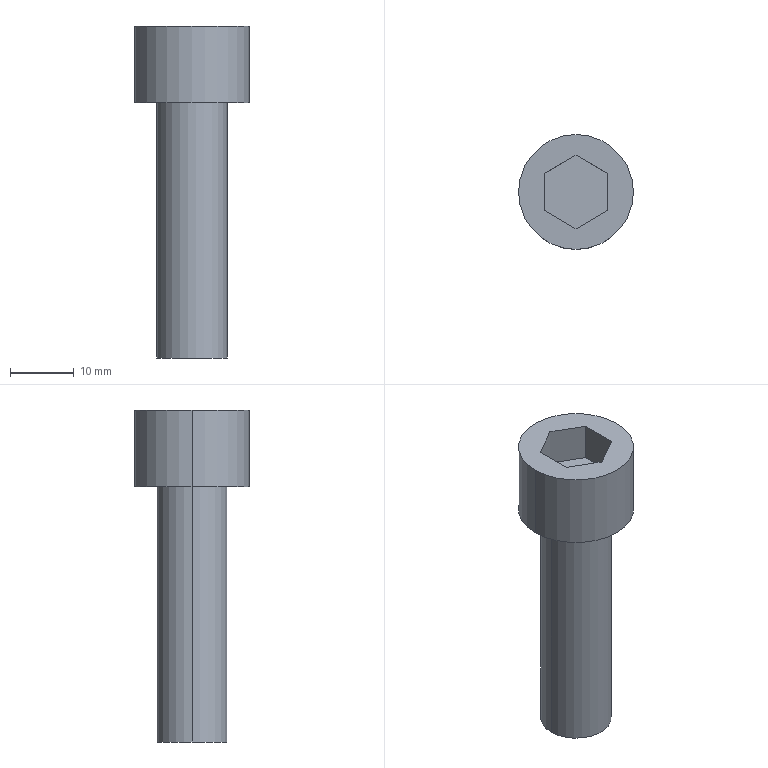Part | SolidWorks | features ICE 2, Extrusion 1 | 1 solid | 14 faces | box 18 x 18 x 52 mm | volume 6335 mm3 | plane 10 | cylinder 4 | commonest cylinder face diameters 11 x2 18 x2
STEP:
#1=CARTESIAN_POINT('',(9.,0.,52.));
#2=VERTEX_POINT('',#1);
#3=CARTESIAN_POINT('',(-9.,0.,52.));
#4=VERTEX_POINT('',#3);
#5=CARTESIAN_POINT('',(0.,0.,52.));
#6=DIRECTION('',(0.,0.,1.));
#7=DIRECTION('',(1.,0.,0.));
#8=AXIS2_PLACEMENT_3D('',#5,#6,#7);
#9=CIRCLE('',#8,9.);
#10=EDGE_CURVE('',#2,#4,#9,.T.);
#11=ORIENTED_EDGE('',*,*,#10,.F.);
#12=CARTESIAN_POINT('',(9.,0.,40.));
#13=VERTEX_POINT('',#12);
#14=CARTESIAN_POINT('',(9.,0.,52.));
#15=DIRECTION('',(0.,0.,-1.));
#16=VECTOR('',#15,1000.);
#17=LINE('',#14,#16);
#18=EDGE_CURVE('',#2,#13,#17,.T.);
#19=ORIENTED_EDGE('',*,*,#18,.T.);
#20=CARTESIAN_POINT('',(-9.,0.,40.));
#21=VERTEX_POINT('',#20);
#22=CARTESIAN_POINT('',(0.,0.,40.));
#23=DIRECTION('',(0.,0.,1.));
#24=DIRECTION('',(1.,0.,0.));
#25=AXIS2_PLACEMENT_3D('',#22,#23,#24);
#26=CIRCLE('',#25,9.);
#27=EDGE_CURVE('',#13,#21,#26,.T.);
#28=ORIENTED_EDGE('',*,*,#27,.T.);
#29=CARTESIAN_POINT('',(-9.,0.,52.));
#30=DIRECTION('',(0.,0.,-1.));
#31=VECTOR('',#30,1000.);
#32=LINE('',#29,#31);
#33=EDGE_CURVE('',#4,#21,#32,.T.);
#34=ORIENTED_EDGE('',*,*,#33,.F.);
#35=EDGE_LOOP('',(#11,#19,#28,#34));
#36=FACE_OUTER_BOUND('',#35,.T.);
#37=CARTESIAN_POINT('',(0.,0.,52.));
#38=DIRECTION('',(0.,0.,-1.));
#39=DIRECTION('',(-1.,0.,0.));
#40=AXIS2_PLACEMENT_3D('',#37,#38,#39);
#41=CYLINDRICAL_SURFACE('',#40,9.);
#42=ADVANCED_FACE('',(#36),#41,.T.);
#43=CARTESIAN_POINT('',(5.5,0.,40.));
#44=VERTEX_POINT('',#43);
#45=CARTESIAN_POINT('',(-5.5,0.,40.));
#46=VERTEX_POINT('',#45);
#47=CARTESIAN_POINT('',(0.,0.,40.));
#48=DIRECTION('',(0.,0.,1.));
#49=DIRECTION('',(1.,0.,0.));
#50=AXIS2_PLACEMENT_3D('',#47,#48,#49);
#51=CIRCLE('',#50,5.5);
#52=EDGE_CURVE('',#44,#46,#51,.T.);
#53=ORIENTED_EDGE('',*,*,#52,.F.);
#54=CARTESIAN_POINT('',(5.5,0.,0.));
#55=VERTEX_POINT('',#54);
#56=CARTESIAN_POINT('',(5.5,0.,40.));
#57=DIRECTION('',(0.,0.,-1.));
#58=VECTOR('',#57,1000.);
#59=LINE('',#56,#58);
#60=EDGE_CURVE('',#44,#55,#59,.T.);
#61=ORIENTED_EDGE('',*,*,#60,.T.);
#62=CARTESIAN_POINT('',(-5.5,0.,0.));
#63=VERTEX_POINT('',#62);
#64=CARTESIAN_POINT('',(0.,0.,0.));
#65=DIRECTION('',(0.,0.,1.));
#66=DIRECTION('',(1.,0.,0.));
#67=AXIS2_PLACEMENT_3D('',#64,#65,#66);
#68=CIRCLE('',#67,5.5);
#69=EDGE_CURVE('',#55,#63,#68,.T.);
#70=ORIENTED_EDGE('',*,*,#69,.T.);
#71=CARTESIAN_POINT('',(-5.5,0.,40.));
#72=DIRECTION('',(0.,0.,-1.));
#73=VECTOR('',#72,1000.);
#74=LINE('',#71,#73);
#75=EDGE_CURVE('',#46,#63,#74,.T.);
#76=ORIENTED_EDGE('',*,*,#75,.F.);
#77=EDGE_LOOP('',(#53,#61,#70,#76));
#78=FACE_OUTER_BOUND('',#77,.T.);
#79=CARTESIAN_POINT('',(0.,0.,40.));
#80=DIRECTION('',(0.,0.,-1.));
#81=DIRECTION('',(-1.,0.,0.));
#82=AXIS2_PLACEMENT_3D('',#79,#80,#81);
#83=CYLINDRICAL_SURFACE('',#82,5.5);
#84=ADVANCED_FACE('',(#78),#83,.T.);
#85=ORIENTED_EDGE('',*,*,#60,.F.);
#86=CARTESIAN_POINT('',(0.,0.,40.));
#87=DIRECTION('',(0.,0.,1.));
#88=DIRECTION('',(1.,0.,0.));
#89=AXIS2_PLACEMENT_3D('',#86,#87,#88);
#90=CIRCLE('',#89,5.5);
#91=EDGE_CURVE('',#46,#44,#90,.T.);
#92=ORIENTED_EDGE('',*,*,#91,.F.);
#93=ORIENTED_EDGE('',*,*,#75,.T.);
#94=CARTESIAN_POINT('',(0.,0.,0.));
#95=DIRECTION('',(0.,0.,1.));
#96=DIRECTION('',(1.,0.,0.));
#97=AXIS2_PLACEMENT_3D('',#94,#95,#96);
#98=CIRCLE('',#97,5.5);
#99=EDGE_CURVE('',#63,#55,#98,.T.);
#100=ORIENTED_EDGE('',*,*,#99,.T.);
#101=EDGE_LOOP('',(#85,#92,#93,#100));
#102=FACE_OUTER_BOUND('',#101,.T.);
#103=CARTESIAN_POINT('',(0.,0.,40.));
#104=DIRECTION('',(0.,0.,-1.));
#105=DIRECTION('',(-1.,0.,0.));
#106=AXIS2_PLACEMENT_3D('',#103,#104,#105);
#107=CYLINDRICAL_SURFACE('',#106,5.5);
#108=ADVANCED_FACE('',(#102),#107,.T.);
#109=ORIENTED_EDGE('',*,*,#99,.F.);
#110=ORIENTED_EDGE('',*,*,#69,.F.);
#111=EDGE_LOOP('',(#109,#110));
#112=FACE_OUTER_BOUND('',#111,.T.);
#113=CARTESIAN_POINT('',(0.,0.,0.));
#114=DIRECTION('',(0.,0.,1.));
#115=DIRECTION('',(1.,0.,0.));
#116=AXIS2_PLACEMENT_3D('',#113,#114,#115);
#117=PLANE('',#116);
#118=ADVANCED_FACE('',(#112),#117,.F.);
#119=CARTESIAN_POINT('',(0.,0.,40.));
#120=DIRECTION('',(0.,0.,1.));
#121=DIRECTION('',(1.,0.,0.));
#122=AXIS2_PLACEMENT_3D('',#119,#120,#121);
#123=CIRCLE('',#122,9.);
#124=EDGE_CURVE('',#21,#13,#123,.T.);
#125=ORIENTED_EDGE('',*,*,#124,.F.);
#126=ORIENTED_EDGE('',*,*,#27,.F.);
#127=EDGE_LOOP('',(#125,#126));
#128=FACE_OUTER_BOUND('',#127,.T.);
#129=ORIENTED_EDGE('',*,*,#91,.T.);
#130=ORIENTED_EDGE('',*,*,#52,.T.);
#131=EDGE_LOOP('',(#129,#130));
#132=FACE_BOUND('',#131,.T.);
#133=CARTESIAN_POINT('',(0.,0.,40.));
#134=DIRECTION('',(0.,0.,1.));
#135=DIRECTION('',(1.,0.,0.));
#136=AXIS2_PLACEMENT_3D('',#133,#134,#135);
#137=PLANE('',#136);
#138=ADVANCED_FACE('',(#128,#132),#137,.F.);
#139=ORIENTED_EDGE('',*,*,#18,.F.);
#140=CARTESIAN_POINT('',(0.,0.,52.));
#141=DIRECTION('',(0.,0.,1.));
#142=DIRECTION('',(1.,0.,0.));
#143=AXIS2_PLACEMENT_3D('',#140,#141,#142);
#144=CIRCLE('',#143,9.);
#145=EDGE_CURVE('',#4,#2,#144,.T.);
#146=ORIENTED_EDGE('',*,*,#145,.F.);
#147=ORIENTED_EDGE('',*,*,#33,.T.);
#148=ORIENTED_EDGE('',*,*,#124,.T.);
#149=EDGE_LOOP('',(#139,#146,#147,#148));
#150=FACE_OUTER_BOUND('',#149,.T.);
#151=CARTESIAN_POINT('',(0.,0.,52.));
#152=DIRECTION('',(0.,0.,-1.));
#153=DIRECTION('',(-1.,0.,0.));
#154=AXIS2_PLACEMENT_3D('',#151,#152,#153);
#155=CYLINDRICAL_SURFACE('',#154,9.);
#156=ADVANCED_FACE('',(#150),#155,.T.);
#157=CARTESIAN_POINT('',(5.,2.887,52.));
#158=VERTEX_POINT('',#157);
#159=CARTESIAN_POINT('',(0.,5.774,52.));
#160=VERTEX_POINT('',#159);
#161=CARTESIAN_POINT('',(5.,2.887,52.));
#162=DIRECTION('',(-0.866,0.5,0.));
#163=VECTOR('',#162,1000.);
#164=LINE('',#161,#163);
#165=EDGE_CURVE('',#158,#160,#164,.T.);
#166=ORIENTED_EDGE('',*,*,#165,.F.);
#167=CARTESIAN_POINT('',(5.,-2.887,52.));
#168=VERTEX_POINT('',#167);
#169=CARTESIAN_POINT('',(5.,-2.887,52.));
#170=DIRECTION('',(0.,1.,0.));
#171=VECTOR('',#170,1000.);
#172=LINE('',#169,#171);
#173=EDGE_CURVE('',#168,#158,#172,.T.);
#174=ORIENTED_EDGE('',*,*,#173,.F.);
#175=CARTESIAN_POINT('',(0.,-5.774,52.));
#176=VERTEX_POINT('',#175);
#177=CARTESIAN_POINT('',(0.,-5.774,52.));
#178=DIRECTION('',(0.866,0.5,0.));
#179=VECTOR('',#178,1000.);
#180=LINE('',#177,#179);
#181=EDGE_CURVE('',#176,#168,#180,.T.);
#182=ORIENTED_EDGE('',*,*,#181,.F.);
#183=CARTESIAN_POINT('',(-5.,-2.887,52.));
#184=VERTEX_POINT('',#183);
#185=CARTESIAN_POINT('',(-5.,-2.887,52.));
#186=DIRECTION('',(0.866,-0.5,0.));
#187=VECTOR('',#186,1000.);
#188=LINE('',#185,#187);
#189=EDGE_CURVE('',#184,#176,#188,.T.);
#190=ORIENTED_EDGE('',*,*,#189,.F.);
#191=CARTESIAN_POINT('',(-5.,2.887,52.));
#192=VERTEX_POINT('',#191);
#193=CARTESIAN_POINT('',(-5.,2.887,52.));
#194=DIRECTION('',(0.,-1.,0.));
#195=VECTOR('',#194,1000.);
#196=LINE('',#193,#195);
#197=EDGE_CURVE('',#192,#184,#196,.T.);
#198=ORIENTED_EDGE('',*,*,#197,.F.);
#199=CARTESIAN_POINT('',(0.,5.774,52.));
#200=DIRECTION('',(-0.866,-0.5,0.));
#201=VECTOR('',#200,1000.);
#202=LINE('',#199,#201);
#203=EDGE_CURVE('',#160,#192,#202,.T.);
#204=ORIENTED_EDGE('',*,*,#203,.F.);
#205=EDGE_LOOP('',(#166,#174,#182,#190,#198,#204));
#206=FACE_BOUND('',#205,.T.);
#207=ORIENTED_EDGE('',*,*,#145,.T.);
#208=ORIENTED_EDGE('',*,*,#10,.T.);
#209=EDGE_LOOP('',(#207,#208));
#210=FACE_OUTER_BOUND('',#209,.T.);
#211=CARTESIAN_POINT('',(0.,0.,52.));
#212=DIRECTION('',(0.,0.,1.));
#213=DIRECTION('',(1.,0.,0.));
#214=AXIS2_PLACEMENT_3D('',#211,#212,#213);
#215=PLANE('',#214);
#216=ADVANCED_FACE('',(#206,#210),#215,.T.);
#217=ORIENTED_EDGE('',*,*,#165,.T.);
#218=CARTESIAN_POINT('',(0.,5.774,46.));
#219=VERTEX_POINT('',#218);
#220=CARTESIAN_POINT('',(0.,5.774,46.));
#221=DIRECTION('',(0.,0.,1.));
#222=VECTOR('',#221,1000.);
#223=LINE('',#220,#222);
#224=EDGE_CURVE('',#219,#160,#223,.T.);
#225=ORIENTED_EDGE('',*,*,#224,.F.);
#226=CARTESIAN_POINT('',(5.,2.887,46.));
#227=VERTEX_POINT('',#226);
#228=CARTESIAN_POINT('',(5.,2.887,46.));
#229=DIRECTION('',(-0.866,0.5,0.));
#230=VECTOR('',#229,1000.);
#231=LINE('',#228,#230);
#232=EDGE_CURVE('',#227,#219,#231,.T.);
#233=ORIENTED_EDGE('',*,*,#232,.F.);
#234=CARTESIAN_POINT('',(5.,2.887,46.));
#235=DIRECTION('',(0.,0.,1.));
#236=VECTOR('',#235,1000.);
#237=LINE('',#234,#236);
#238=EDGE_CURVE('',#227,#158,#237,.T.);
#239=ORIENTED_EDGE('',*,*,#238,.T.);
#240=EDGE_LOOP('',(#217,#225,#233,#239));
#241=FACE_OUTER_BOUND('',#240,.T.);
#242=CARTESIAN_POINT('',(5.,2.887,46.));
#243=DIRECTION('',(0.5,0.866,0.));
#244=DIRECTION('',(-0.866,0.5,0.));
#245=AXIS2_PLACEMENT_3D('',#242,#243,#244);
#246=PLANE('',#245);
#247=ADVANCED_FACE('',(#241),#246,.F.);
#248=ORIENTED_EDGE('',*,*,#173,.T.);
#249=ORIENTED_EDGE('',*,*,#238,.F.);
#250=CARTESIAN_POINT('',(5.,-2.887,46.));
#251=VERTEX_POINT('',#250);
#252=CARTESIAN_POINT('',(5.,-2.887,46.));
#253=DIRECTION('',(0.,1.,0.));
#254=VECTOR('',#253,1000.);
#255=LINE('',#252,#254);
#256=EDGE_CURVE('',#251,#227,#255,.T.);
#257=ORIENTED_EDGE('',*,*,#256,.F.);
#258=CARTESIAN_POINT('',(5.,-2.887,46.));
#259=DIRECTION('',(0.,0.,1.));
#260=VECTOR('',#259,1000.);
#261=LINE('',#258,#260);
#262=EDGE_CURVE('',#251,#168,#261,.T.);
#263=ORIENTED_EDGE('',*,*,#262,.T.);
#264=EDGE_LOOP('',(#248,#249,#257,#263));
#265=FACE_OUTER_BOUND('',#264,.T.);
#266=CARTESIAN_POINT('',(5.,-2.887,46.));
#267=DIRECTION('',(1.,0.,0.));
#268=DIRECTION('',(0.,1.,0.));
#269=AXIS2_PLACEMENT_3D('',#266,#267,#268);
#270=PLANE('',#269);
#271=ADVANCED_FACE('',(#265),#270,.F.);
#272=ORIENTED_EDGE('',*,*,#181,.T.);
#273=ORIENTED_EDGE('',*,*,#262,.F.);
#274=CARTESIAN_POINT('',(0.,-5.774,46.));
#275=VERTEX_POINT('',#274);
#276=CARTESIAN_POINT('',(0.,-5.774,46.));
#277=DIRECTION('',(0.866,0.5,0.));
#278=VECTOR('',#277,1000.);
#279=LINE('',#276,#278);
#280=EDGE_CURVE('',#275,#251,#279,.T.);
#281=ORIENTED_EDGE('',*,*,#280,.F.);
#282=CARTESIAN_POINT('',(0.,-5.774,46.));
#283=DIRECTION('',(0.,0.,1.));
#284=VECTOR('',#283,1000.);
#285=LINE('',#282,#284);
#286=EDGE_CURVE('',#275,#176,#285,.T.);
#287=ORIENTED_EDGE('',*,*,#286,.T.);
#288=EDGE_LOOP('',(#272,#273,#281,#287));
#289=FACE_OUTER_BOUND('',#288,.T.);
#290=CARTESIAN_POINT('',(0.,-5.774,46.));
#291=DIRECTION('',(0.5,-0.866,0.));
#292=DIRECTION('',(0.866,0.5,0.));
#293=AXIS2_PLACEMENT_3D('',#290,#291,#292);
#294=PLANE('',#293);
#295=ADVANCED_FACE('',(#289),#294,.F.);
#296=ORIENTED_EDGE('',*,*,#189,.T.);
#297=ORIENTED_EDGE('',*,*,#286,.F.);
#298=CARTESIAN_POINT('',(-5.,-2.887,46.));
#299=VERTEX_POINT('',#298);
#300=CARTESIAN_POINT('',(-5.,-2.887,46.));
#301=DIRECTION('',(0.866,-0.5,0.));
#302=VECTOR('',#301,1000.);
#303=LINE('',#300,#302);
#304=EDGE_CURVE('',#299,#275,#303,.T.);
#305=ORIENTED_EDGE('',*,*,#304,.F.);
#306=CARTESIAN_POINT('',(-5.,-2.887,46.));
#307=DIRECTION('',(0.,0.,1.));
#308=VECTOR('',#307,1000.);
#309=LINE('',#306,#308);
#310=EDGE_CURVE('',#299,#184,#309,.T.);
#311=ORIENTED_EDGE('',*,*,#310,.T.);
#312=EDGE_LOOP('',(#296,#297,#305,#311));
#313=FACE_OUTER_BOUND('',#312,.T.);
#314=CARTESIAN_POINT('',(-5.,-2.887,46.));
#315=DIRECTION('',(-0.5,-0.866,0.));
#316=DIRECTION('',(0.866,-0.5,0.));
#317=AXIS2_PLACEMENT_3D('',#314,#315,#316);
#318=PLANE('',#317);
#319=ADVANCED_FACE('',(#313),#318,.F.);
#320=ORIENTED_EDGE('',*,*,#197,.T.);
#321=ORIENTED_EDGE('',*,*,#310,.F.);
#322=CARTESIAN_POINT('',(-5.,2.887,46.));
#323=VERTEX_POINT('',#322);
#324=CARTESIAN_POINT('',(-5.,2.887,46.));
#325=DIRECTION('',(0.,-1.,0.));
#326=VECTOR('',#325,1000.);
#327=LINE('',#324,#326);
#328=EDGE_CURVE('',#323,#299,#327,.T.);
#329=ORIENTED_EDGE('',*,*,#328,.F.);
#330=CARTESIAN_POINT('',(-5.,2.887,46.));
#331=DIRECTION('',(0.,0.,1.));
#332=VECTOR('',#331,1000.);
#333=LINE('',#330,#332);
#334=EDGE_CURVE('',#323,#192,#333,.T.);
#335=ORIENTED_EDGE('',*,*,#334,.T.);
#336=EDGE_LOOP('',(#320,#321,#329,#335));
#337=FACE_OUTER_BOUND('',#336,.T.);
#338=CARTESIAN_POINT('',(-5.,2.887,46.));
#339=DIRECTION('',(-1.,0.,0.));
#340=DIRECTION('',(0.,0.,1.));
#341=AXIS2_PLACEMENT_3D('',#338,#339,#340);
#342=PLANE('',#341);
#343=ADVANCED_FACE('',(#337),#342,.F.);
#344=ORIENTED_EDGE('',*,*,#203,.T.);
#345=ORIENTED_EDGE('',*,*,#334,.F.);
#346=CARTESIAN_POINT('',(0.,5.774,46.));
#347=DIRECTION('',(-0.866,-0.5,0.));
#348=VECTOR('',#347,1000.);
#349=LINE('',#346,#348);
#350=EDGE_CURVE('',#219,#323,#349,.T.);
#351=ORIENTED_EDGE('',*,*,#350,.F.);
#352=ORIENTED_EDGE('',*,*,#224,.T.);
#353=EDGE_LOOP('',(#344,#345,#351,#352));
#354=FACE_OUTER_BOUND('',#353,.T.);
#355=CARTESIAN_POINT('',(0.,5.774,46.));
#356=DIRECTION('',(-0.5,0.866,0.));
#357=DIRECTION('',(-0.866,-0.5,0.));
#358=AXIS2_PLACEMENT_3D('',#355,#356,#357);
#359=PLANE('',#358);
#360=ADVANCED_FACE('',(#354),#359,.F.);
#361=ORIENTED_EDGE('',*,*,#232,.T.);
#362=ORIENTED_EDGE('',*,*,#350,.T.);
#363=ORIENTED_EDGE('',*,*,#328,.T.);
#364=ORIENTED_EDGE('',*,*,#304,.T.);
#365=ORIENTED_EDGE('',*,*,#280,.T.);
#366=ORIENTED_EDGE('',*,*,#256,.T.);
#367=EDGE_LOOP('',(#361,#362,#363,#364,#365,#366));
#368=FACE_OUTER_BOUND('',#367,.T.);
#369=CARTESIAN_POINT('',(0.,0.,46.));
#370=DIRECTION('',(0.,0.,1.));
#371=DIRECTION('',(1.,0.,0.));
#372=AXIS2_PLACEMENT_3D('',#369,#370,#371);
#373=PLANE('',#372);
#374=ADVANCED_FACE('',(#368),#373,.T.);
#375=CLOSED_SHELL('',(#42,#84,#108,#118,#138,#156,#216,#247,#271,#295,#319,#343,#360,#374));
#376=MANIFOLD_SOLID_BREP('',#375);
#377=CARTESIAN_POINT('',(0.,0.,0.));
#378=DIRECTION('',(0.,0.,1.));
#379=DIRECTION('',(1.,0.,0.));
#380=AXIS2_PLACEMENT_3D('',#377,#378,#379);
#381=(LENGTH_UNIT()NAMED_UNIT(*)SI_UNIT(.MILLI.,.METRE.));
#382=UNCERTAINTY_MEASURE_WITH_UNIT(LENGTH_MEASURE(0.00001),#381,'','');
#383=(NAMED_UNIT(*)PLANE_ANGLE_UNIT()SI_UNIT($,.RADIAN.));
#384=(NAMED_UNIT(*)SI_UNIT($,.STERADIAN.)SOLID_ANGLE_UNIT());
#385=(GEOMETRIC_REPRESENTATION_CONTEXT(3)GLOBAL_UNCERTAINTY_ASSIGNED_CONTEXT((#382))GLOBAL_UNIT_ASSIGNED_CONTEXT((#381,#383,#384))REPRESENTATION_CONTEXT('',''));
#386=ADVANCED_BREP_SHAPE_REPRESENTATION('',(#376,#380),#385);